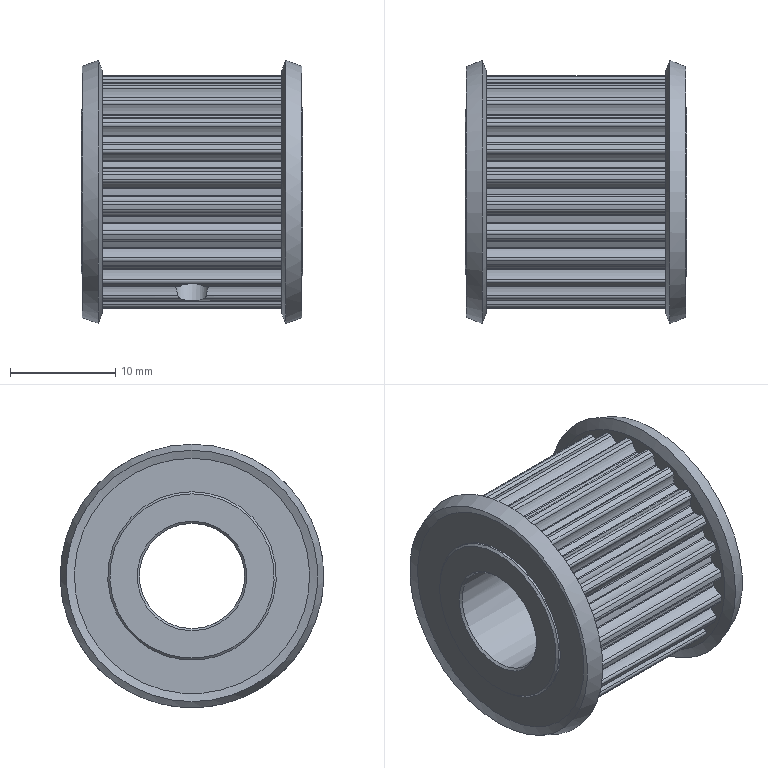Part | NX | 1 solid | 225 faces | box 21 x 25 x 25 mm | volume 5815 mm3 | cylinder 211 | cone 8 | plane 6 | commonest cylinder face diameters 0.3 x52 0.56 x52 3.95 x52 19.94 x26 22.16 x24 3.242 x2